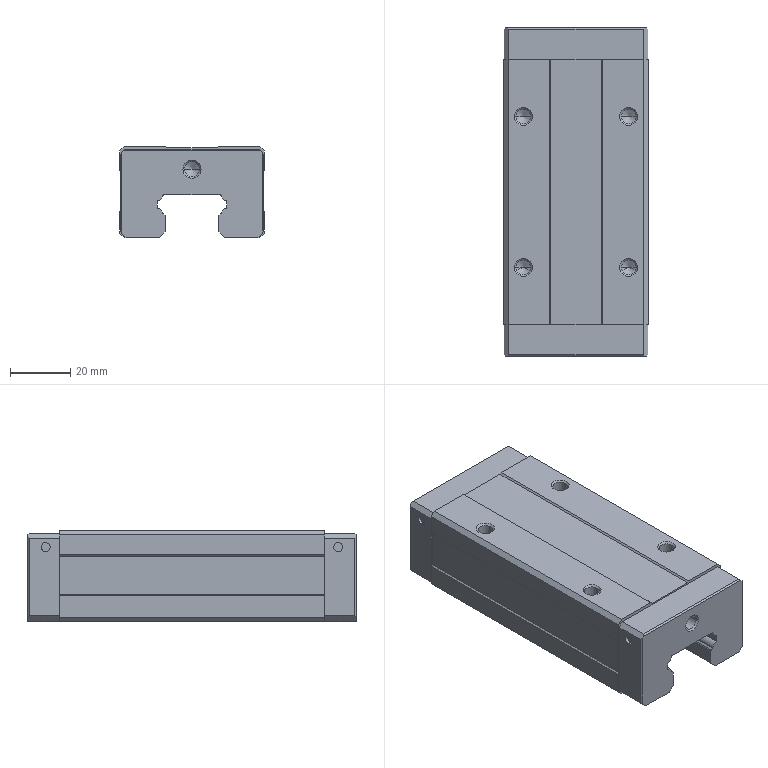Part | 1 solid | 126 faces | box 48 x 109 x 30.2 mm | volume 123162 mm3 | plane 66 | cylinder 36 | cone 24 | commonest cylinder face diameters 4.917 x12 3 x8 0.6 x4 0.594 x2 0.985 x2 0.988 x2